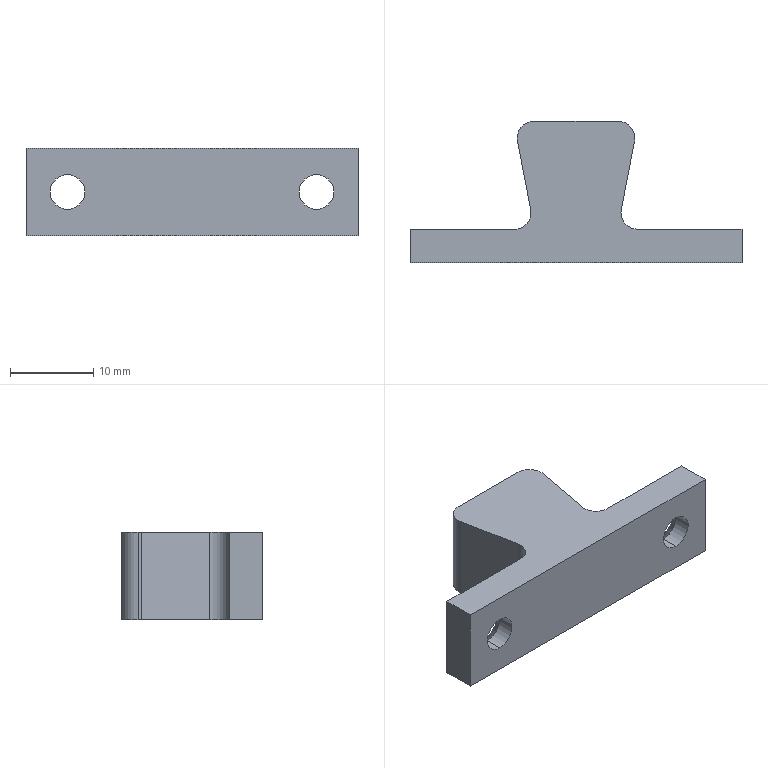Part | STEP file | Ball catch 2 | 1 solid | 24 faces | box 40 x 17 x 10.5 mm | volume 3213 mm3 | cylinder 10 | plane 10 | cone 4 | commonest cylinder face diameters 4 x6 4.2 x4